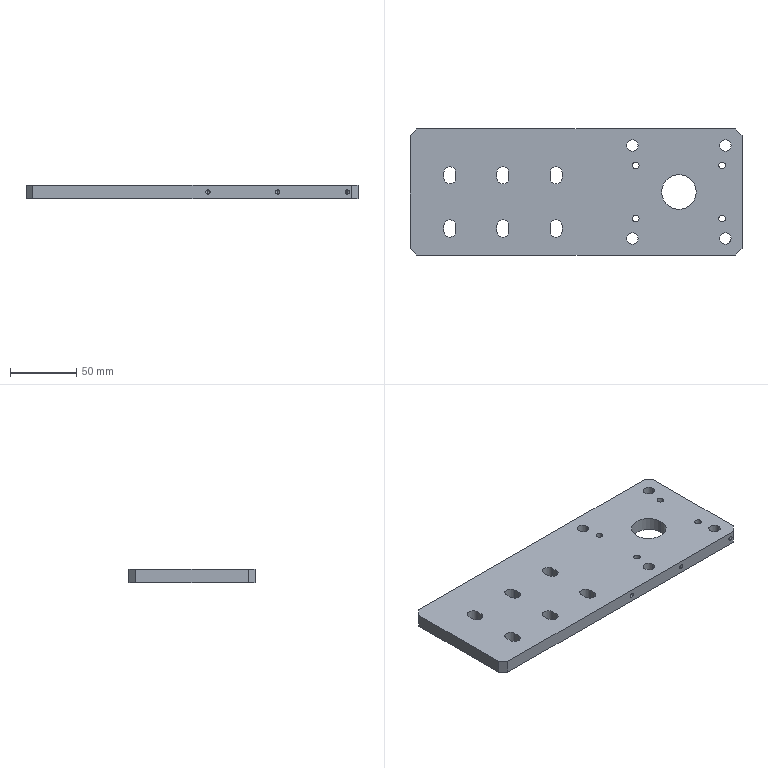Part | SolidWorks | features 3DProfileFeature 4, HoleWzd 4, ICE 2, LPattern 2, Chamfer 1, Extrusion 1 | 1 solid | 64 faces | box 250 x 95 x 10 mm | volume 222392 mm3 | cylinder 36 | plane 22 | cone 6 | commonest cylinder face diameters 9 x12 5 x8 8.5 x8 3.3 x6 26 x2